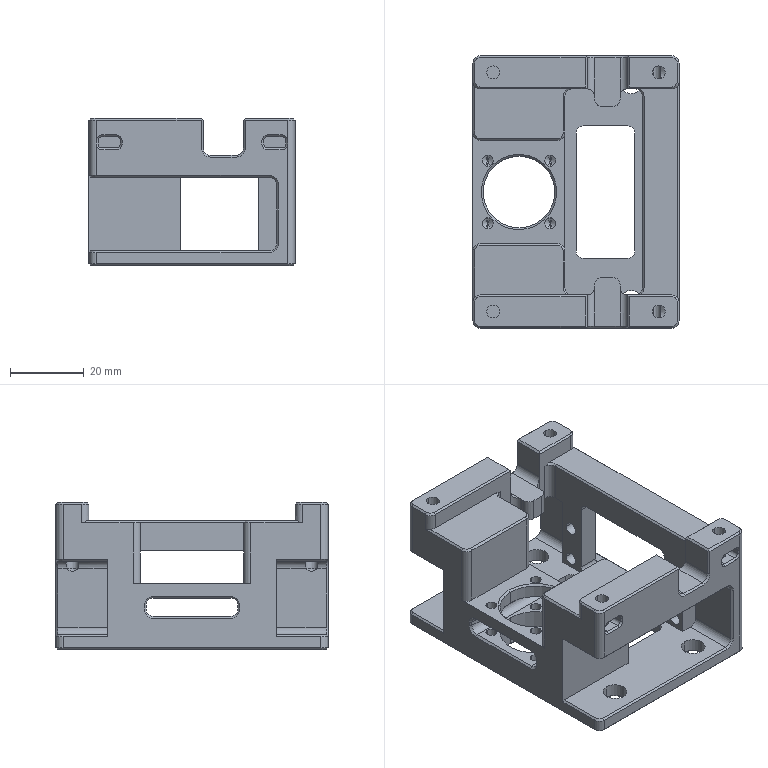Part | 1 solid | 357 faces | box 56 x 74 x 40 mm | volume 54679 mm3 | plane 151 | cylinder 120 | cone 86 | commonest cylinder face diameters 4 x52 3.5 x24 2 x16 3 x16 6.5 x8 19.5 x4